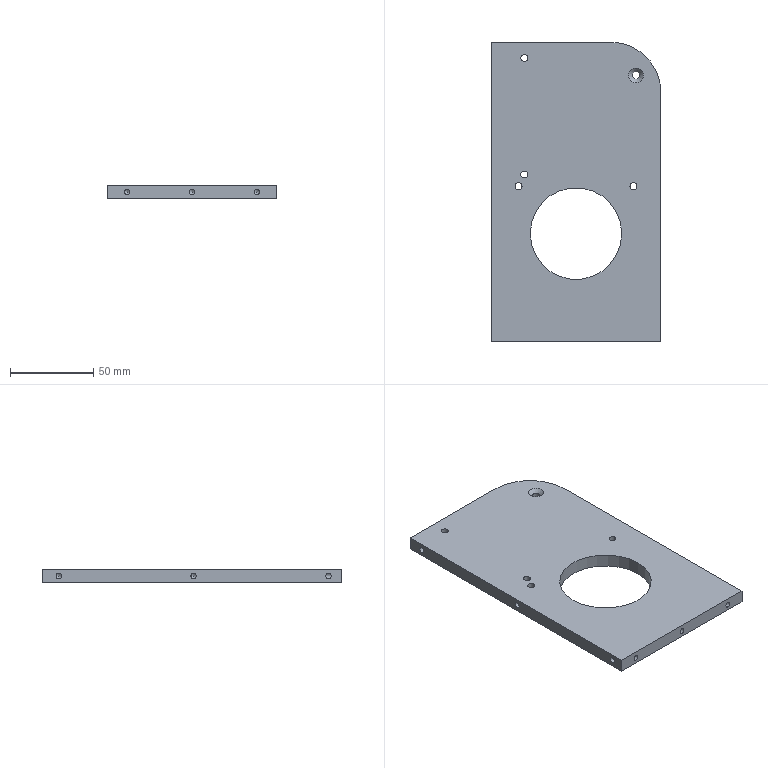Part | NX | 1 solid | 36 faces | box 102 x 180 x 8 mm | volume 124761 mm3 | cylinder 18 | cone 12 | plane 6 | commonest cylinder face diameters 3.3 x11 4.2 x4 4.5 x1 55 x1 60 x1
STEP:
#1=CARTESIAN_POINT('',(39.5,-130.5,-1.572));
#2=VERTEX_POINT('',#1);
#3=CARTESIAN_POINT('',(39.5,-129.5,-1.572));
#4=VERTEX_POINT('',#3);
#5=CARTESIAN_POINT('',(39.5,-130.,0.));
#6=DIRECTION('',(1.,0.,0.));
#7=DIRECTION('',(0.,0.,-1.));
#8=AXIS2_PLACEMENT_3D('',#5,#6,#7);
#9=CIRCLE('',#8,1.65);
#10=EDGE_CURVE('',#2,#4,#9,.T.);
#11=ORIENTED_EDGE('',*,*,#10,.T.);
#12=CARTESIAN_POINT('',(39.5,-129.5,-1.572));
#13=CARTESIAN_POINT('',(39.449,-129.829,-1.589));
#14=CARTESIAN_POINT('',(39.449,-130.17,-1.589));
#15=CARTESIAN_POINT('',(39.5,-130.5,-1.572));
#16=B_SPLINE_CURVE_WITH_KNOTS('',3,(#12,#13,#14,#15),.UNSPECIFIED.,.F.,.F.,(4,4),(0.000476,0.001477),.UNSPECIFIED.);
#17=EDGE_CURVE('',#4,#2,#16,.T.);
#18=ORIENTED_EDGE('',*,*,#17,.T.);
#19=EDGE_LOOP('',(#11,#18));
#20=FACE_BOUND('',#19,.T.);
#21=CARTESIAN_POINT('',(39.5,-130.,0.));
#22=DIRECTION('',(1.,0.,0.));
#23=DIRECTION('',(0.,0.,-1.));
#24=AXIS2_PLACEMENT_3D('',#21,#22,#23);
#25=CONICAL_SURFACE('',#24,1.65,1.03);
#26=ADVANCED_FACE('',(#20),#25,.F.);
#27=CARTESIAN_POINT('',(-39.5,-132.5,1.572));
#28=VERTEX_POINT('',#27);
#29=CARTESIAN_POINT('',(-39.5,-131.5,1.572));
#30=VERTEX_POINT('',#29);
#31=CARTESIAN_POINT('',(-39.5,-132.,0.));
#32=DIRECTION('',(-1.,0.,0.));
#33=DIRECTION('',(0.,0.,1.));
#34=AXIS2_PLACEMENT_3D('',#31,#32,#33);
#35=CIRCLE('',#34,1.65);
#36=EDGE_CURVE('',#28,#30,#35,.T.);
#37=ORIENTED_EDGE('',*,*,#36,.T.);
#38=CARTESIAN_POINT('',(-39.5,-131.5,1.572));
#39=CARTESIAN_POINT('',(-39.449,-131.829,1.589));
#40=CARTESIAN_POINT('',(-39.449,-132.17,1.589));
#41=CARTESIAN_POINT('',(-39.5,-132.5,1.572));
#42=B_SPLINE_CURVE_WITH_KNOTS('',3,(#38,#39,#40,#41),.UNSPECIFIED.,.F.,.F.,(4,4),(0.000476,0.001477),.UNSPECIFIED.);
#43=EDGE_CURVE('',#30,#28,#42,.T.);
#44=ORIENTED_EDGE('',*,*,#43,.T.);
#45=EDGE_LOOP('',(#37,#44));
#46=FACE_BOUND('',#45,.T.);
#47=CARTESIAN_POINT('',(-39.5,-132.,0.));
#48=DIRECTION('',(-1.,0.,0.));
#49=DIRECTION('',(0.,0.,1.));
#50=AXIS2_PLACEMENT_3D('',#47,#48,#49);
#51=CONICAL_SURFACE('',#50,1.65,1.03);
#52=ADVANCED_FACE('',(#46),#51,.F.);
#53=CARTESIAN_POINT('',(-28.9,30.505,4.));
#54=VERTEX_POINT('',#53);
#55=CARTESIAN_POINT('',(-31.,30.505,4.));
#56=DIRECTION('',(0.,0.,1.));
#57=DIRECTION('',(1.,0.,0.));
#58=AXIS2_PLACEMENT_3D('',#55,#56,#57);
#59=CIRCLE('',#58,2.1);
#60=EDGE_CURVE('',#54,#54,#59,.T.);
#61=ORIENTED_EDGE('',*,*,#60,.F.);
#62=EDGE_LOOP('',(#61));
#63=FACE_BOUND('',#62,.T.);
#64=CARTESIAN_POINT('',(-28.9,-39.495,4.));
#65=VERTEX_POINT('',#64);
#66=CARTESIAN_POINT('',(-31.,-39.495,4.));
#67=DIRECTION('',(0.,0.,1.));
#68=DIRECTION('',(1.,0.,0.));
#69=AXIS2_PLACEMENT_3D('',#66,#67,#68);
#70=CIRCLE('',#69,2.1);
#71=EDGE_CURVE('',#65,#65,#70,.T.);
#72=ORIENTED_EDGE('',*,*,#71,.F.);
#73=EDGE_LOOP('',(#72));
#74=FACE_BOUND('',#73,.T.);
#75=CARTESIAN_POINT('',(36.6,-46.5,4.));
#76=VERTEX_POINT('',#75);
#77=CARTESIAN_POINT('',(34.5,-46.5,4.));
#78=DIRECTION('',(0.,0.,1.));
#79=DIRECTION('',(1.,0.,0.));
#80=AXIS2_PLACEMENT_3D('',#77,#78,#79);
#81=CIRCLE('',#80,2.1);
#82=EDGE_CURVE('',#76,#76,#81,.T.);
#83=ORIENTED_EDGE('',*,*,#82,.F.);
#84=EDGE_LOOP('',(#83));
#85=FACE_BOUND('',#84,.T.);
#86=CARTESIAN_POINT('',(-32.4,-46.5,4.));
#87=VERTEX_POINT('',#86);
#88=CARTESIAN_POINT('',(-34.5,-46.5,4.));
#89=DIRECTION('',(0.,0.,1.));
#90=DIRECTION('',(1.,0.,0.));
#91=AXIS2_PLACEMENT_3D('',#88,#89,#90);
#92=CIRCLE('',#91,2.1);
#93=EDGE_CURVE('',#87,#87,#92,.T.);
#94=ORIENTED_EDGE('',*,*,#93,.F.);
#95=EDGE_LOOP('',(#94));
#96=FACE_BOUND('',#95,.T.);
#97=CARTESIAN_POINT('',(40.5,20.,4.));
#98=VERTEX_POINT('',#97);
#99=CARTESIAN_POINT('',(36.,20.,4.));
#100=DIRECTION('',(0.,0.,1.));
#101=DIRECTION('',(1.,0.,0.));
#102=AXIS2_PLACEMENT_3D('',#99,#100,#101);
#103=CIRCLE('',#102,4.5);
#104=EDGE_CURVE('',#98,#98,#103,.T.);
#105=ORIENTED_EDGE('',*,*,#104,.F.);
#106=EDGE_LOOP('',(#105));
#107=FACE_BOUND('',#106,.T.);
#108=CARTESIAN_POINT('',(51.,-140.,4.));
#109=VERTEX_POINT('',#108);
#110=CARTESIAN_POINT('',(51.,10.,4.));
#111=VERTEX_POINT('',#110);
#112=CARTESIAN_POINT('',(51.,40.,4.));
#113=DIRECTION('',(0.,1.,0.));
#114=VECTOR('',#113,1000.);
#115=LINE('',#112,#114);
#116=EDGE_CURVE('',#109,#111,#115,.T.);
#117=ORIENTED_EDGE('',*,*,#116,.T.);
#118=CARTESIAN_POINT('',(21.,40.,4.));
#119=VERTEX_POINT('',#118);
#120=CARTESIAN_POINT('',(21.,10.,4.));
#121=DIRECTION('',(0.,0.,1.));
#122=DIRECTION('',(1.,0.,0.));
#123=AXIS2_PLACEMENT_3D('',#120,#121,#122);
#124=CIRCLE('',#123,30.);
#125=EDGE_CURVE('',#111,#119,#124,.T.);
#126=ORIENTED_EDGE('',*,*,#125,.T.);
#127=CARTESIAN_POINT('',(-51.,40.,4.));
#128=VERTEX_POINT('',#127);
#129=CARTESIAN_POINT('',(-51.,40.,4.));
#130=DIRECTION('',(-1.,0.,0.));
#131=VECTOR('',#130,1000.);
#132=LINE('',#129,#131);
#133=EDGE_CURVE('',#119,#128,#132,.T.);
#134=ORIENTED_EDGE('',*,*,#133,.T.);
#135=CARTESIAN_POINT('',(-51.,-140.,4.));
#136=VERTEX_POINT('',#135);
#137=CARTESIAN_POINT('',(-51.,40.,4.));
#138=DIRECTION('',(0.,-1.,0.));
#139=VECTOR('',#138,1000.);
#140=LINE('',#137,#139);
#141=EDGE_CURVE('',#128,#136,#140,.T.);
#142=ORIENTED_EDGE('',*,*,#141,.T.);
#143=CARTESIAN_POINT('',(51.,-140.,4.));
#144=DIRECTION('',(-1.,0.,0.));
#145=VECTOR('',#144,1000.);
#146=LINE('',#143,#145);
#147=EDGE_CURVE('',#109,#136,#146,.T.);
#148=ORIENTED_EDGE('',*,*,#147,.F.);
#149=EDGE_LOOP('',(#117,#126,#134,#142,#148));
#150=FACE_BOUND('',#149,.T.);
#151=CARTESIAN_POINT('',(-27.5,-75.,4.));
#152=VERTEX_POINT('',#151);
#153=CARTESIAN_POINT('',(0.,-75.,4.));
#154=DIRECTION('',(0.,0.,-1.));
#155=DIRECTION('',(-1.,0.,0.));
#156=AXIS2_PLACEMENT_3D('',#153,#154,#155);
#157=CIRCLE('',#156,27.5);
#158=EDGE_CURVE('',#152,#152,#157,.T.);
#159=ORIENTED_EDGE('',*,*,#158,.T.);
#160=EDGE_LOOP('',(#159));
#161=FACE_BOUND('',#160,.T.);
#162=CARTESIAN_POINT('',(0.,0.,4.));
#163=DIRECTION('',(0.,0.,1.));
#164=DIRECTION('',(1.,0.,0.));
#165=AXIS2_PLACEMENT_3D('',#162,#163,#164);
#166=PLANE('',#165);
#167=ADVANCED_FACE('',(#63,#74,#85,#96,#107,#150,#161),#166,.T.);
#168=CARTESIAN_POINT('',(-28.9,30.505,-4.));
#169=VERTEX_POINT('',#168);
#170=CARTESIAN_POINT('',(-31.,30.505,-4.));
#171=DIRECTION('',(0.,0.,1.));
#172=DIRECTION('',(1.,0.,0.));
#173=AXIS2_PLACEMENT_3D('',#170,#171,#172);
#174=CIRCLE('',#173,2.1);
#175=EDGE_CURVE('',#169,#169,#174,.T.);
#176=ORIENTED_EDGE('',*,*,#175,.T.);
#177=EDGE_LOOP('',(#176));
#178=FACE_BOUND('',#177,.T.);
#179=CARTESIAN_POINT('',(-28.9,-39.495,-4.));
#180=VERTEX_POINT('',#179);
#181=CARTESIAN_POINT('',(-31.,-39.495,-4.));
#182=DIRECTION('',(0.,0.,1.));
#183=DIRECTION('',(1.,0.,0.));
#184=AXIS2_PLACEMENT_3D('',#181,#182,#183);
#185=CIRCLE('',#184,2.1);
#186=EDGE_CURVE('',#180,#180,#185,.T.);
#187=ORIENTED_EDGE('',*,*,#186,.T.);
#188=EDGE_LOOP('',(#187));
#189=FACE_BOUND('',#188,.T.);
#190=CARTESIAN_POINT('',(36.6,-46.5,-4.));
#191=VERTEX_POINT('',#190);
#192=CARTESIAN_POINT('',(34.5,-46.5,-4.));
#193=DIRECTION('',(0.,0.,1.));
#194=DIRECTION('',(1.,0.,0.));
#195=AXIS2_PLACEMENT_3D('',#192,#193,#194);
#196=CIRCLE('',#195,2.1);
#197=EDGE_CURVE('',#191,#191,#196,.T.);
#198=ORIENTED_EDGE('',*,*,#197,.T.);
#199=EDGE_LOOP('',(#198));
#200=FACE_BOUND('',#199,.T.);
#201=CARTESIAN_POINT('',(-32.4,-46.5,-4.));
#202=VERTEX_POINT('',#201);
#203=CARTESIAN_POINT('',(-34.5,-46.5,-4.));
#204=DIRECTION('',(0.,0.,1.));
#205=DIRECTION('',(1.,0.,0.));
#206=AXIS2_PLACEMENT_3D('',#203,#204,#205);
#207=CIRCLE('',#206,2.1);
#208=EDGE_CURVE('',#202,#202,#207,.T.);
#209=ORIENTED_EDGE('',*,*,#208,.T.);
#210=EDGE_LOOP('',(#209));
#211=FACE_BOUND('',#210,.T.);
#212=CARTESIAN_POINT('',(38.25,20.,-4.));
#213=VERTEX_POINT('',#212);
#214=CARTESIAN_POINT('',(36.,20.,-4.));
#215=DIRECTION('',(0.,0.,1.));
#216=DIRECTION('',(1.,0.,0.));
#217=AXIS2_PLACEMENT_3D('',#214,#215,#216);
#218=CIRCLE('',#217,2.25);
#219=EDGE_CURVE('',#213,#213,#218,.T.);
#220=ORIENTED_EDGE('',*,*,#219,.T.);
#221=EDGE_LOOP('',(#220));
#222=FACE_BOUND('',#221,.T.);
#223=CARTESIAN_POINT('',(21.,40.,-4.));
#224=VERTEX_POINT('',#223);
#225=CARTESIAN_POINT('',(-51.,40.,-4.));
#226=VERTEX_POINT('',#225);
#227=CARTESIAN_POINT('',(-51.,40.,-4.));
#228=DIRECTION('',(-1.,0.,0.));
#229=VECTOR('',#228,1000.);
#230=LINE('',#227,#229);
#231=EDGE_CURVE('',#224,#226,#230,.T.);
#232=ORIENTED_EDGE('',*,*,#231,.F.);
#233=CARTESIAN_POINT('',(51.,10.,-4.));
#234=VERTEX_POINT('',#233);
#235=CARTESIAN_POINT('',(21.,10.,-4.));
#236=DIRECTION('',(0.,0.,1.));
#237=DIRECTION('',(1.,0.,0.));
#238=AXIS2_PLACEMENT_3D('',#235,#236,#237);
#239=CIRCLE('',#238,30.);
#240=EDGE_CURVE('',#224,#234,#239,.F.);
#241=ORIENTED_EDGE('',*,*,#240,.T.);
#242=CARTESIAN_POINT('',(51.,-140.,-4.));
#243=VERTEX_POINT('',#242);
#244=CARTESIAN_POINT('',(51.,40.,-4.));
#245=DIRECTION('',(0.,1.,0.));
#246=VECTOR('',#245,1000.);
#247=LINE('',#244,#246);
#248=EDGE_CURVE('',#243,#234,#247,.T.);
#249=ORIENTED_EDGE('',*,*,#248,.F.);
#250=CARTESIAN_POINT('',(-51.,-140.,-4.));
#251=VERTEX_POINT('',#250);
#252=CARTESIAN_POINT('',(51.,-140.,-4.));
#253=DIRECTION('',(1.,0.,0.));
#254=VECTOR('',#253,1000.);
#255=LINE('',#252,#254);
#256=EDGE_CURVE('',#251,#243,#255,.T.);
#257=ORIENTED_EDGE('',*,*,#256,.F.);
#258=CARTESIAN_POINT('',(-51.,40.,-4.));
#259=DIRECTION('',(0.,-1.,0.));
#260=VECTOR('',#259,1000.);
#261=LINE('',#258,#260);
#262=EDGE_CURVE('',#226,#251,#261,.T.);
#263=ORIENTED_EDGE('',*,*,#262,.F.);
#264=EDGE_LOOP('',(#232,#241,#249,#257,#263));
#265=FACE_BOUND('',#264,.T.);
#266=CARTESIAN_POINT('',(-27.5,-75.,-4.));
#267=VERTEX_POINT('',#266);
#268=CARTESIAN_POINT('',(0.,-75.,-4.));
#269=DIRECTION('',(0.,0.,-1.));
#270=DIRECTION('',(-1.,0.,0.));
#271=AXIS2_PLACEMENT_3D('',#268,#269,#270);
#272=CIRCLE('',#271,27.5);
#273=EDGE_CURVE('',#267,#267,#272,.T.);
#274=ORIENTED_EDGE('',*,*,#273,.F.);
#275=EDGE_LOOP('',(#274));
#276=FACE_BOUND('',#275,.T.);
#277=CARTESIAN_POINT('',(0.,0.,-4.));
#278=DIRECTION('',(0.,0.,1.));
#279=DIRECTION('',(1.,0.,0.));
#280=AXIS2_PLACEMENT_3D('',#277,#278,#279);
#281=PLANE('',#280);
#282=ADVANCED_FACE('',(#178,#189,#200,#211,#222,#265,#276),#281,.F.);
#283=CARTESIAN_POINT('',(51.,5.,-1.65));
#284=VERTEX_POINT('',#283);
#285=CARTESIAN_POINT('',(51.,5.,0.));
#286=DIRECTION('',(1.,0.,0.));
#287=DIRECTION('',(0.,0.,-1.));
#288=AXIS2_PLACEMENT_3D('',#285,#286,#287);
#289=CIRCLE('',#288,1.65);
#290=EDGE_CURVE('',#284,#284,#289,.T.);
#291=ORIENTED_EDGE('',*,*,#290,.F.);
#292=EDGE_LOOP('',(#291));
#293=FACE_BOUND('',#292,.T.);
#294=CARTESIAN_POINT('',(51.,-130.,-1.65));
#295=VERTEX_POINT('',#294);
#296=CARTESIAN_POINT('',(51.,-130.,0.));
#297=DIRECTION('',(1.,0.,0.));
#298=DIRECTION('',(0.,0.,-1.));
#299=AXIS2_PLACEMENT_3D('',#296,#297,#298);
#300=CIRCLE('',#299,1.65);
#301=EDGE_CURVE('',#295,#295,#300,.T.);
#302=ORIENTED_EDGE('',*,*,#301,.F.);
#303=EDGE_LOOP('',(#302));
#304=FACE_BOUND('',#303,.T.);
#305=ORIENTED_EDGE('',*,*,#248,.T.);
#306=CARTESIAN_POINT('',(51.,10.,4.));
#307=DIRECTION('',(0.,0.,-1.));
#308=VECTOR('',#307,1000.);
#309=LINE('',#306,#308);
#310=EDGE_CURVE('',#234,#111,#309,.F.);
#311=ORIENTED_EDGE('',*,*,#310,.T.);
#312=ORIENTED_EDGE('',*,*,#116,.F.);
#313=CARTESIAN_POINT('',(51.,-140.,-146.843));
#314=DIRECTION('',(0.,0.,1.));
#315=VECTOR('',#314,1000.);
#316=LINE('',#313,#315);
#317=EDGE_CURVE('',#243,#109,#316,.T.);
#318=ORIENTED_EDGE('',*,*,#317,.F.);
#319=EDGE_LOOP('',(#305,#311,#312,#318));
#320=FACE_BOUND('',#319,.T.);
#321=CARTESIAN_POINT('',(51.,40.,4.));
#322=DIRECTION('',(-1.,0.,0.));
#323=DIRECTION('',(0.,0.,1.));
#324=AXIS2_PLACEMENT_3D('',#321,#322,#323);
#325=PLANE('',#324);
#326=ADVANCED_FACE('',(#293,#304,#320),#325,.F.);
#327=CARTESIAN_POINT('',(-31.,40.,1.65));
#328=VERTEX_POINT('',#327);
#329=CARTESIAN_POINT('',(-31.,40.,0.));
#330=DIRECTION('',(0.,1.,0.));
#331=DIRECTION('',(0.,0.,1.));
#332=AXIS2_PLACEMENT_3D('',#329,#330,#331);
#333=CIRCLE('',#332,1.65);
#334=EDGE_CURVE('',#328,#328,#333,.T.);
#335=ORIENTED_EDGE('',*,*,#334,.F.);
#336=EDGE_LOOP('',(#335));
#337=FACE_BOUND('',#336,.T.);
#338=ORIENTED_EDGE('',*,*,#133,.F.);
#339=CARTESIAN_POINT('',(21.,40.,4.));
#340=DIRECTION('',(0.,0.,-1.));
#341=VECTOR('',#340,1000.);
#342=LINE('',#339,#341);
#343=EDGE_CURVE('',#119,#224,#342,.T.);
#344=ORIENTED_EDGE('',*,*,#343,.T.);
#345=ORIENTED_EDGE('',*,*,#231,.T.);
#346=CARTESIAN_POINT('',(-51.,40.,4.));
#347=DIRECTION('',(0.,0.,-1.));
#348=VECTOR('',#347,1000.);
#349=LINE('',#346,#348);
#350=EDGE_CURVE('',#128,#226,#349,.T.);
#351=ORIENTED_EDGE('',*,*,#350,.F.);
#352=EDGE_LOOP('',(#338,#344,#345,#351));
#353=FACE_BOUND('',#352,.T.);
#354=CARTESIAN_POINT('',(-51.,40.,4.));
#355=DIRECTION('',(0.,-1.,0.));
#356=DIRECTION('',(0.,0.,-1.));
#357=AXIS2_PLACEMENT_3D('',#354,#355,#356);
#358=PLANE('',#357);
#359=ADVANCED_FACE('',(#337,#353),#358,.F.);
#360=CARTESIAN_POINT('',(-51.,30.,1.65));
#361=VERTEX_POINT('',#360);
#362=CARTESIAN_POINT('',(-51.,30.,0.));
#363=DIRECTION('',(-1.,0.,0.));
#364=DIRECTION('',(0.,0.,1.));
#365=AXIS2_PLACEMENT_3D('',#362,#363,#364);
#366=CIRCLE('',#365,1.65);
#367=EDGE_CURVE('',#361,#361,#366,.T.);
#368=ORIENTED_EDGE('',*,*,#367,.F.);
#369=EDGE_LOOP('',(#368));
#370=FACE_BOUND('',#369,.T.);
#371=CARTESIAN_POINT('',(-51.,-51.,1.65));
#372=VERTEX_POINT('',#371);
#373=CARTESIAN_POINT('',(-51.,-51.,0.));
#374=DIRECTION('',(-1.,0.,0.));
#375=DIRECTION('',(0.,0.,1.));
#376=AXIS2_PLACEMENT_3D('',#373,#374,#375);
#377=CIRCLE('',#376,1.65);
#378=EDGE_CURVE('',#372,#372,#377,.T.);
#379=ORIENTED_EDGE('',*,*,#378,.F.);
#380=EDGE_LOOP('',(#379));
#381=FACE_BOUND('',#380,.T.);
#382=CARTESIAN_POINT('',(-51.,-132.,1.65));
#383=VERTEX_POINT('',#382);
#384=CARTESIAN_POINT('',(-51.,-132.,0.));
#385=DIRECTION('',(-1.,0.,0.));
#386=DIRECTION('',(0.,0.,1.));
#387=AXIS2_PLACEMENT_3D('',#384,#385,#386);
#388=CIRCLE('',#387,1.65);
#389=EDGE_CURVE('',#383,#383,#388,.T.);
#390=ORIENTED_EDGE('',*,*,#389,.F.);
#391=EDGE_LOOP('',(#390));
#392=FACE_BOUND('',#391,.T.);
#393=ORIENTED_EDGE('',*,*,#262,.T.);
#394=CARTESIAN_POINT('',(-51.,-140.,-146.843));
#395=DIRECTION('',(0.,0.,1.));
#396=VECTOR('',#395,1000.);
#397=LINE('',#394,#396);
#398=EDGE_CURVE('',#251,#136,#397,.T.);
#399=ORIENTED_EDGE('',*,*,#398,.T.);
#400=ORIENTED_EDGE('',*,*,#141,.F.);
#401=ORIENTED_EDGE('',*,*,#350,.T.);
#402=EDGE_LOOP('',(#393,#399,#400,#401));
#403=FACE_BOUND('',#402,.T.);
#404=CARTESIAN_POINT('',(-51.,40.,4.));
#405=DIRECTION('',(1.,0.,0.));
#406=DIRECTION('',(0.,1.,0.));
#407=AXIS2_PLACEMENT_3D('',#404,#405,#406);
#408=PLANE('',#407);
#409=ADVANCED_FACE('',(#370,#381,#392,#403),#408,.F.);
#410=CARTESIAN_POINT('',(39.,-140.,-1.65));
#411=VERTEX_POINT('',#410);
#412=CARTESIAN_POINT('',(39.,-140.,0.));
#413=DIRECTION('',(0.,-1.,0.));
#414=DIRECTION('',(0.,0.,-1.));
#415=AXIS2_PLACEMENT_3D('',#412,#413,#414);
#416=CIRCLE('',#415,1.65);
#417=EDGE_CURVE('',#411,#411,#416,.T.);
#418=ORIENTED_EDGE('',*,*,#417,.F.);
#419=EDGE_LOOP('',(#418));
#420=FACE_BOUND('',#419,.T.);
#421=CARTESIAN_POINT('',(0.,-140.,-1.65));
#422=VERTEX_POINT('',#421);
#423=CARTESIAN_POINT('',(0.,-140.,0.));
#424=DIRECTION('',(0.,-1.,0.));
#425=DIRECTION('',(0.,0.,-1.));
#426=AXIS2_PLACEMENT_3D('',#423,#424,#425);
#427=CIRCLE('',#426,1.65);
#428=EDGE_CURVE('',#422,#422,#427,.T.);
#429=ORIENTED_EDGE('',*,*,#428,.F.);
#430=EDGE_LOOP('',(#429));
#431=FACE_BOUND('',#430,.T.);
#432=CARTESIAN_POINT('',(-39.,-140.,-1.65));
#433=VERTEX_POINT('',#432);
#434=CARTESIAN_POINT('',(-39.,-140.,0.));
#435=DIRECTION('',(0.,-1.,0.));
#436=DIRECTION('',(0.,0.,-1.));
#437=AXIS2_PLACEMENT_3D('',#434,#435,#436);
#438=CIRCLE('',#437,1.65);
#439=EDGE_CURVE('',#433,#433,#438,.T.);
#440=ORIENTED_EDGE('',*,*,#439,.F.);
#441=EDGE_LOOP('',(#440));
#442=FACE_BOUND('',#441,.T.);
#443=ORIENTED_EDGE('',*,*,#398,.F.);
#444=ORIENTED_EDGE('',*,*,#256,.T.);
#445=ORIENTED_EDGE('',*,*,#317,.T.);
#446=ORIENTED_EDGE('',*,*,#147,.T.);
#447=EDGE_LOOP('',(#443,#444,#445,#446));
#448=FACE_BOUND('',#447,.T.);
#449=CARTESIAN_POINT('',(51.,-140.,-146.843));
#450=DIRECTION('',(0.,1.,0.));
#451=DIRECTION('',(0.,0.,1.));
#452=AXIS2_PLACEMENT_3D('',#449,#450,#451);
#453=PLANE('',#452);
#454=ADVANCED_FACE('',(#420,#431,#442,#448),#453,.F.);
#455=ORIENTED_EDGE('',*,*,#273,.T.);
#456=EDGE_LOOP('',(#455));
#457=FACE_BOUND('',#456,.T.);
#458=ORIENTED_EDGE('',*,*,#158,.F.);
#459=EDGE_LOOP('',(#458));
#460=FACE_BOUND('',#459,.T.);
#461=CARTESIAN_POINT('',(0.,-75.,-4.));
#462=DIRECTION('',(0.,0.,1.));
#463=DIRECTION('',(1.,0.,0.));
#464=AXIS2_PLACEMENT_3D('',#461,#462,#463);
#465=CYLINDRICAL_SURFACE('',#464,27.5);
#466=ADVANCED_FACE('',(#457,#460),#465,.F.);
#467=CARTESIAN_POINT('',(-39.5,-131.5,-1.572));
#468=VERTEX_POINT('',#467);
#469=CARTESIAN_POINT('',(-39.5,-132.5,-1.572));
#470=VERTEX_POINT('',#469);
#471=CARTESIAN_POINT('',(-39.5,-132.,0.));
#472=DIRECTION('',(-1.,0.,0.));
#473=DIRECTION('',(0.,0.,1.));
#474=AXIS2_PLACEMENT_3D('',#471,#472,#473);
#475=CIRCLE('',#474,1.65);
#476=EDGE_CURVE('',#468,#470,#475,.T.);
#477=ORIENTED_EDGE('',*,*,#476,.T.);
#478=CARTESIAN_POINT('',(-39.5,-132.5,-1.572));
#479=CARTESIAN_POINT('',(-39.449,-132.171,-1.589));
#480=CARTESIAN_POINT('',(-39.449,-131.83,-1.589));
#481=CARTESIAN_POINT('',(-39.5,-131.5,-1.572));
#482=B_SPLINE_CURVE_WITH_KNOTS('',3,(#478,#479,#480,#481),.UNSPECIFIED.,.F.,.F.,(4,4),(0.000476,0.001477),.UNSPECIFIED.);
#483=EDGE_CURVE('',#470,#468,#482,.T.);
#484=ORIENTED_EDGE('',*,*,#483,.T.);
#485=EDGE_LOOP('',(#477,#484));
#486=FACE_BOUND('',#485,.T.);
#487=CARTESIAN_POINT('',(-39.5,-132.,0.));
#488=DIRECTION('',(-1.,0.,0.));
#489=DIRECTION('',(0.,0.,1.));
#490=AXIS2_PLACEMENT_3D('',#487,#488,#489);
#491=CONICAL_SURFACE('',#490,1.65,1.03);
#492=ADVANCED_FACE('',(#486),#491,.F.);
#493=ORIENTED_EDGE('',*,*,#476,.F.);
#494=CARTESIAN_POINT('',(-39.,-132.,0.));
#495=DIRECTION('',(-0.7071,-0.7071,0.));
#496=DIRECTION('',(-0.7071,0.7071,0.));
#497=AXIS2_PLACEMENT_3D('',#494,#495,#496);
#498=ELLIPSE('',#497,2.333,1.65);
#499=EDGE_CURVE('',#468,#30,#498,.F.);
#500=ORIENTED_EDGE('',*,*,#499,.T.);
#501=ORIENTED_EDGE('',*,*,#36,.F.);
#502=CARTESIAN_POINT('',(-39.,-132.,0.));
#503=DIRECTION('',(-0.7071,0.7071,0.));
#504=DIRECTION('',(-0.7071,-0.7071,0.));
#505=AXIS2_PLACEMENT_3D('',#502,#503,#504);
#506=ELLIPSE('',#505,2.333,1.65);
#507=EDGE_CURVE('',#28,#470,#506,.F.);
#508=ORIENTED_EDGE('',*,*,#507,.T.);
#509=EDGE_LOOP('',(#493,#500,#501,#508));
#510=FACE_BOUND('',#509,.T.);
#511=ORIENTED_EDGE('',*,*,#389,.T.);
#512=EDGE_LOOP('',(#511));
#513=FACE_BOUND('',#512,.T.);
#514=CARTESIAN_POINT('',(-51.,-132.,0.));
#515=DIRECTION('',(-1.,0.,0.));
#516=DIRECTION('',(0.,0.,1.));
#517=AXIS2_PLACEMENT_3D('',#514,#515,#516);
#518=CYLINDRICAL_SURFACE('',#517,1.65);
#519=ADVANCED_FACE('',(#510,#513),#518,.F.);
#520=CARTESIAN_POINT('',(-38.509,-51.,0.));
#521=VERTEX_POINT('',#520);
#522=VERTEX_LOOP('',#521);
#523=FACE_BOUND('',#522,.T.);
#524=CARTESIAN_POINT('',(-39.5,-51.,1.65));
#525=VERTEX_POINT('',#524);
#526=CARTESIAN_POINT('',(-39.5,-51.,0.));
#527=DIRECTION('',(-1.,0.,0.));
#528=DIRECTION('',(0.,0.,1.));
#529=AXIS2_PLACEMENT_3D('',#526,#527,#528);
#530=CIRCLE('',#529,1.65);
#531=EDGE_CURVE('',#525,#525,#530,.T.);
#532=ORIENTED_EDGE('',*,*,#531,.T.);
#533=EDGE_LOOP('',(#532));
#534=FACE_BOUND('',#533,.T.);
#535=CARTESIAN_POINT('',(-39.5,-51.,0.));
#536=DIRECTION('',(-1.,0.,0.));
#537=DIRECTION('',(0.,0.,1.));
#538=AXIS2_PLACEMENT_3D('',#535,#536,#537);
#539=CONICAL_SURFACE('',#538,1.65,1.03);
#540=ADVANCED_FACE('',(#523,#534),#539,.F.);
#541=ORIENTED_EDGE('',*,*,#531,.F.);
#542=EDGE_LOOP('',(#541));
#543=FACE_BOUND('',#542,.T.);
#544=ORIENTED_EDGE('',*,*,#378,.T.);
#545=EDGE_LOOP('',(#544));
#546=FACE_BOUND('',#545,.T.);
#547=CARTESIAN_POINT('',(-51.,-51.,0.));
#548=DIRECTION('',(-1.,0.,0.));
#549=DIRECTION('',(0.,0.,1.));
#550=AXIS2_PLACEMENT_3D('',#547,#548,#549);
#551=CYLINDRICAL_SURFACE('',#550,1.65);
#552=ADVANCED_FACE('',(#543,#546),#551,.F.);
#553=CARTESIAN_POINT('',(-38.509,30.,0.));
#554=VERTEX_POINT('',#553);
#555=VERTEX_LOOP('',#554);
#556=FACE_BOUND('',#555,.T.);
#557=CARTESIAN_POINT('',(-39.5,30.,1.65));
#558=VERTEX_POINT('',#557);
#559=CARTESIAN_POINT('',(-39.5,30.,0.));
#560=DIRECTION('',(-1.,0.,0.));
#561=DIRECTION('',(0.,0.,1.));
#562=AXIS2_PLACEMENT_3D('',#559,#560,#561);
#563=CIRCLE('',#562,1.65);
#564=EDGE_CURVE('',#558,#558,#563,.T.);
#565=ORIENTED_EDGE('',*,*,#564,.T.);
#566=EDGE_LOOP('',(#565));
#567=FACE_BOUND('',#566,.T.);
#568=CARTESIAN_POINT('',(-39.5,30.,0.));
#569=DIRECTION('',(-1.,0.,0.));
#570=DIRECTION('',(0.,0.,1.));
#571=AXIS2_PLACEMENT_3D('',#568,#569,#570);
#572=CONICAL_SURFACE('',#571,1.65,1.03);
#573=ADVANCED_FACE('',(#556,#567),#572,.F.);
#574=ORIENTED_EDGE('',*,*,#564,.F.);
#575=EDGE_LOOP('',(#574));
#576=FACE_BOUND('',#575,.T.);
#577=ORIENTED_EDGE('',*,*,#367,.T.);
#578=EDGE_LOOP('',(#577));
#579=FACE_BOUND('',#578,.T.);
#580=CARTESIAN_POINT('',(-51.,30.,0.));
#581=DIRECTION('',(-1.,0.,0.));
#582=DIRECTION('',(0.,0.,1.));
#583=AXIS2_PLACEMENT_3D('',#580,#581,#582);
#584=CYLINDRICAL_SURFACE('',#583,1.65);
#585=ADVANCED_FACE('',(#576,#579),#584,.F.);
#586=CARTESIAN_POINT('',(-31.,32.605,1.65));
#587=VERTEX_POINT('',#586);
#588=CARTESIAN_POINT('',(-29.691,32.284,1.274));
#589=CARTESIAN_POINT('',(-30.998,32.767,1.844));
#590=CARTESIAN_POINT('',(-32.097,32.36,1.35));
#591=CARTESIAN_POINT('',(-32.549,31.937,0.6794));
#592=CARTESIAN_POINT('',(-32.744,31.677,-0.2313));
#593=CARTESIAN_POINT('',(-32.308,32.285,-1.267));
#594=CARTESIAN_POINT('',(-31.01,32.764,-1.838));
#595=CARTESIAN_POINT('',(-29.693,32.289,-1.281));
#596=CARTESIAN_POINT('',(-29.179,31.563,-0.0006032));
#597=CARTESIAN_POINT('',(-29.691,32.284,1.274));
#598=CARTESIAN_POINT('',(-30.998,32.767,1.844));
#599=CARTESIAN_POINT('',(-32.097,32.36,1.35));
#600=B_SPLINE_CURVE_WITH_KNOTS('',3,(#588,#589,#590,#591,#592,#593,#594,#595,#596,#597,#598,#599),.UNSPECIFIED.,.T.,.F.,(1,1,1,1,1,1,1,1,1,1,1,1,1,1,1,1),(-0.00408,-0.00272,-0.00136,0.,0.00136,0.00204,0.00272,0.00408,0.00544,0.006799,0.008159,0.009519,0.01088,0.01224,0.01292,0.0136),.UNSPECIFIED.);
#601=EDGE_CURVE('',#587,#587,#600,.T.);
#602=ORIENTED_EDGE('',*,*,#601,.T.);
#603=EDGE_LOOP('',(#602));
#604=FACE_BOUND('',#603,.T.);
#605=ORIENTED_EDGE('',*,*,#334,.T.);
#606=EDGE_LOOP('',(#605));
#607=FACE_BOUND('',#606,.T.);
#608=CARTESIAN_POINT('',(-31.,40.,0.));
#609=DIRECTION('',(0.,1.,0.));
#610=DIRECTION('',(0.,0.,1.));
#611=AXIS2_PLACEMENT_3D('',#608,#609,#610);
#612=CYLINDRICAL_SURFACE('',#611,1.65);
#613=ADVANCED_FACE('',(#604,#607),#612,.F.);
#614=CARTESIAN_POINT('',(39.5,-129.5,1.572));
#615=VERTEX_POINT('',#614);
#616=CARTESIAN_POINT('',(39.5,-130.5,1.572));
#617=VERTEX_POINT('',#616);
#618=CARTESIAN_POINT('',(39.5,-130.,0.));
#619=DIRECTION('',(1.,0.,0.));
#620=DIRECTION('',(0.,0.,-1.));
#621=AXIS2_PLACEMENT_3D('',#618,#619,#620);
#622=CIRCLE('',#621,1.65);
#623=EDGE_CURVE('',#615,#617,#622,.T.);
#624=ORIENTED_EDGE('',*,*,#623,.T.);
#625=CARTESIAN_POINT('',(39.5,-130.5,1.572));
#626=CARTESIAN_POINT('',(39.449,-130.171,1.589));
#627=CARTESIAN_POINT('',(39.449,-129.83,1.589));
#628=CARTESIAN_POINT('',(39.5,-129.5,1.572));
#629=B_SPLINE_CURVE_WITH_KNOTS('',3,(#625,#626,#627,#628),.UNSPECIFIED.,.F.,.F.,(4,4),(0.000476,0.001477),.UNSPECIFIED.);
#630=EDGE_CURVE('',#617,#615,#629,.T.);
#631=ORIENTED_EDGE('',*,*,#630,.T.);
#632=EDGE_LOOP('',(#624,#631));
#633=FACE_BOUND('',#632,.T.);
#634=CARTESIAN_POINT('',(39.5,-130.,0.));
#635=DIRECTION('',(1.,0.,0.));
#636=DIRECTION('',(0.,0.,-1.));
#637=AXIS2_PLACEMENT_3D('',#634,#635,#636);
#638=CONICAL_SURFACE('',#637,1.65,1.03);
#639=ADVANCED_FACE('',(#633),#638,.F.);
#640=ORIENTED_EDGE('',*,*,#623,.F.);
#641=CARTESIAN_POINT('',(39.,-130.,0.));
#642=DIRECTION('',(0.7071,-0.7071,0.));
#643=DIRECTION('',(0.7071,0.7071,0.));
#644=AXIS2_PLACEMENT_3D('',#641,#642,#643);
#645=ELLIPSE('',#644,2.333,1.65);
#646=EDGE_CURVE('',#615,#4,#645,.F.);
#647=ORIENTED_EDGE('',*,*,#646,.T.);
#648=ORIENTED_EDGE('',*,*,#10,.F.);
#649=CARTESIAN_POINT('',(39.,-130.,0.));
#650=DIRECTION('',(0.7071,0.7071,0.));
#651=DIRECTION('',(0.7071,-0.7071,0.));
#652=AXIS2_PLACEMENT_3D('',#649,#650,#651);
#653=ELLIPSE('',#652,2.333,1.65);
#654=EDGE_CURVE('',#2,#617,#653,.F.);
#655=ORIENTED_EDGE('',*,*,#654,.T.);
#656=EDGE_LOOP('',(#640,#647,#648,#655));
#657=FACE_BOUND('',#656,.T.);
#658=ORIENTED_EDGE('',*,*,#301,.T.);
#659=EDGE_LOOP('',(#658));
#660=FACE_BOUND('',#659,.T.);
#661=CARTESIAN_POINT('',(51.,-130.,0.));
#662=DIRECTION('',(1.,0.,0.));
#663=DIRECTION('',(0.,0.,-1.));
#664=AXIS2_PLACEMENT_3D('',#661,#662,#663);
#665=CYLINDRICAL_SURFACE('',#664,1.65);
#666=ADVANCED_FACE('',(#657,#660),#665,.F.);
#667=CARTESIAN_POINT('',(38.509,5.,0.));
#668=VERTEX_POINT('',#667);
#669=VERTEX_LOOP('',#668);
#670=FACE_BOUND('',#669,.T.);
#671=CARTESIAN_POINT('',(39.5,5.,-1.65));
#672=VERTEX_POINT('',#671);
#673=CARTESIAN_POINT('',(39.5,5.,0.));
#674=DIRECTION('',(1.,0.,0.));
#675=DIRECTION('',(0.,0.,-1.));
#676=AXIS2_PLACEMENT_3D('',#673,#674,#675);
#677=CIRCLE('',#676,1.65);
#678=EDGE_CURVE('',#672,#672,#677,.T.);
#679=ORIENTED_EDGE('',*,*,#678,.T.);
#680=EDGE_LOOP('',(#679));
#681=FACE_BOUND('',#680,.T.);
#682=CARTESIAN_POINT('',(39.5,5.,0.));
#683=DIRECTION('',(1.,0.,0.));
#684=DIRECTION('',(0.,0.,-1.));
#685=AXIS2_PLACEMENT_3D('',#682,#683,#684);
#686=CONICAL_SURFACE('',#685,1.65,1.03);
#687=ADVANCED_FACE('',(#670,#681),#686,.F.);
#688=ORIENTED_EDGE('',*,*,#678,.F.);
#689=EDGE_LOOP('',(#688));
#690=FACE_BOUND('',#689,.T.);
#691=ORIENTED_EDGE('',*,*,#290,.T.);
#692=EDGE_LOOP('',(#691));
#693=FACE_BOUND('',#692,.T.);
#694=CARTESIAN_POINT('',(51.,5.,0.));
#695=DIRECTION('',(1.,0.,0.));
#696=DIRECTION('',(0.,0.,-1.));
#697=AXIS2_PLACEMENT_3D('',#694,#695,#696);
#698=CYLINDRICAL_SURFACE('',#697,1.65);
#699=ADVANCED_FACE('',(#690,#693),#698,.F.);
#700=ORIENTED_EDGE('',*,*,#439,.T.);
#701=EDGE_LOOP('',(#700));
#702=FACE_BOUND('',#701,.T.);
#703=CARTESIAN_POINT('',(-39.,-125.,-1.65));
#704=VERTEX_POINT('',#703);
#705=CARTESIAN_POINT('',(-39.,-125.,0.));
#706=DIRECTION('',(0.,-1.,0.));
#707=DIRECTION('',(0.,0.,-1.));
#708=AXIS2_PLACEMENT_3D('',#705,#706,#707);
#709=CIRCLE('',#708,1.65);
#710=EDGE_CURVE('',#704,#704,#709,.T.);
#711=ORIENTED_EDGE('',*,*,#710,.F.);
#712=EDGE_LOOP('',(#711));
#713=FACE_BOUND('',#712,.T.);
#714=ORIENTED_EDGE('',*,*,#499,.F.);
#715=ORIENTED_EDGE('',*,*,#483,.F.);
#716=ORIENTED_EDGE('',*,*,#507,.F.);
#717=ORIENTED_EDGE('',*,*,#43,.F.);
#718=EDGE_LOOP('',(#714,#715,#716,#717));
#719=FACE_BOUND('',#718,.T.);
#720=CARTESIAN_POINT('',(-39.,-140.,0.));
#721=DIRECTION('',(0.,-1.,0.));
#722=DIRECTION('',(0.,0.,-1.));
#723=AXIS2_PLACEMENT_3D('',#720,#721,#722);
#724=CYLINDRICAL_SURFACE('',#723,1.65);
#725=ADVANCED_FACE('',(#702,#713,#719),#724,.F.);
#726=CARTESIAN_POINT('',(-39.,-124.009,0.));
#727=VERTEX_POINT('',#726);
#728=VERTEX_LOOP('',#727);
#729=FACE_BOUND('',#728,.T.);
#730=ORIENTED_EDGE('',*,*,#710,.T.);
#731=EDGE_LOOP('',(#730));
#732=FACE_BOUND('',#731,.T.);
#733=CARTESIAN_POINT('',(-39.,-125.,0.));
#734=DIRECTION('',(0.,-1.,0.));
#735=DIRECTION('',(0.,0.,-1.));
#736=AXIS2_PLACEMENT_3D('',#733,#734,#735);
#737=CONICAL_SURFACE('',#736,1.65,1.03);
#738=ADVANCED_FACE('',(#729,#732),#737,.F.);
#739=CARTESIAN_POINT('',(0.,-124.009,0.));
#740=VERTEX_POINT('',#739);
#741=VERTEX_LOOP('',#740);
#742=FACE_BOUND('',#741,.T.);
#743=CARTESIAN_POINT('',(0.,-125.,-1.65));
#744=VERTEX_POINT('',#743);
#745=CARTESIAN_POINT('',(0.,-125.,0.));
#746=DIRECTION('',(0.,-1.,0.));
#747=DIRECTION('',(0.,0.,-1.));
#748=AXIS2_PLACEMENT_3D('',#745,#746,#747);
#749=CIRCLE('',#748,1.65);
#750=EDGE_CURVE('',#744,#744,#749,.T.);
#751=ORIENTED_EDGE('',*,*,#750,.T.);
#752=EDGE_LOOP('',(#751));
#753=FACE_BOUND('',#752,.T.);
#754=CARTESIAN_POINT('',(0.,-125.,0.));
#755=DIRECTION('',(0.,-1.,0.));
#756=DIRECTION('',(0.,0.,-1.));
#757=AXIS2_PLACEMENT_3D('',#754,#755,#756);
#758=CONICAL_SURFACE('',#757,1.65,1.03);
#759=ADVANCED_FACE('',(#742,#753),#758,.F.);
#760=ORIENTED_EDGE('',*,*,#750,.F.);
#761=EDGE_LOOP('',(#760));
#762=FACE_BOUND('',#761,.T.);
#763=ORIENTED_EDGE('',*,*,#428,.T.);
#764=EDGE_LOOP('',(#763));
#765=FACE_BOUND('',#764,.T.);
#766=CARTESIAN_POINT('',(0.,-140.,0.));
#767=DIRECTION('',(0.,-1.,0.));
#768=DIRECTION('',(0.,0.,-1.));
#769=AXIS2_PLACEMENT_3D('',#766,#767,#768);
#770=CYLINDRICAL_SURFACE('',#769,1.65);
#771=ADVANCED_FACE('',(#762,#765),#770,.F.);
#772=ORIENTED_EDGE('',*,*,#417,.T.);
#773=EDGE_LOOP('',(#772));
#774=FACE_BOUND('',#773,.T.);
#775=CARTESIAN_POINT('',(39.,-125.,-1.65));
#776=VERTEX_POINT('',#775);
#777=CARTESIAN_POINT('',(39.,-125.,0.));
#778=DIRECTION('',(0.,-1.,0.));
#779=DIRECTION('',(0.,0.,-1.));
#780=AXIS2_PLACEMENT_3D('',#777,#778,#779);
#781=CIRCLE('',#780,1.65);
#782=EDGE_CURVE('',#776,#776,#781,.T.);
#783=ORIENTED_EDGE('',*,*,#782,.F.);
#784=EDGE_LOOP('',(#783));
#785=FACE_BOUND('',#784,.T.);
#786=ORIENTED_EDGE('',*,*,#646,.F.);
#787=ORIENTED_EDGE('',*,*,#630,.F.);
#788=ORIENTED_EDGE('',*,*,#654,.F.);
#789=ORIENTED_EDGE('',*,*,#17,.F.);
#790=EDGE_LOOP('',(#786,#787,#788,#789));
#791=FACE_BOUND('',#790,.T.);
#792=CARTESIAN_POINT('',(39.,-140.,0.));
#793=DIRECTION('',(0.,-1.,0.));
#794=DIRECTION('',(0.,0.,-1.));
#795=AXIS2_PLACEMENT_3D('',#792,#793,#794);
#796=CYLINDRICAL_SURFACE('',#795,1.65);
#797=ADVANCED_FACE('',(#774,#785,#791),#796,.F.);
#798=CARTESIAN_POINT('',(39.,-124.009,0.));
#799=VERTEX_POINT('',#798);
#800=VERTEX_LOOP('',#799);
#801=FACE_BOUND('',#800,.T.);
#802=ORIENTED_EDGE('',*,*,#782,.T.);
#803=EDGE_LOOP('',(#802));
#804=FACE_BOUND('',#803,.T.);
#805=CARTESIAN_POINT('',(39.,-125.,0.));
#806=DIRECTION('',(0.,-1.,0.));
#807=DIRECTION('',(0.,0.,-1.));
#808=AXIS2_PLACEMENT_3D('',#805,#806,#807);
#809=CONICAL_SURFACE('',#808,1.65,1.03);
#810=ADVANCED_FACE('',(#801,#804),#809,.F.);
#811=ORIENTED_EDGE('',*,*,#219,.F.);
#812=EDGE_LOOP('',(#811));
#813=FACE_BOUND('',#812,.T.);
#814=CARTESIAN_POINT('',(38.25,20.,1.75));
#815=VERTEX_POINT('',#814);
#816=CARTESIAN_POINT('',(36.,20.,1.75));
#817=DIRECTION('',(0.,0.,1.));
#818=DIRECTION('',(1.,0.,0.));
#819=AXIS2_PLACEMENT_3D('',#816,#817,#818);
#820=CIRCLE('',#819,2.25);
#821=EDGE_CURVE('',#815,#815,#820,.T.);
#822=ORIENTED_EDGE('',*,*,#821,.T.);
#823=EDGE_LOOP('',(#822));
#824=FACE_BOUND('',#823,.T.);
#825=CARTESIAN_POINT('',(36.,20.,4.));
#826=DIRECTION('',(0.,0.,1.));
#827=DIRECTION('',(1.,0.,0.));
#828=AXIS2_PLACEMENT_3D('',#825,#826,#827);
#829=CYLINDRICAL_SURFACE('',#828,2.25);
#830=ADVANCED_FACE('',(#813,#824),#829,.F.);
#831=ORIENTED_EDGE('',*,*,#821,.F.);
#832=EDGE_LOOP('',(#831));
#833=FACE_BOUND('',#832,.T.);
#834=ORIENTED_EDGE('',*,*,#104,.T.);
#835=EDGE_LOOP('',(#834));
#836=FACE_BOUND('',#835,.T.);
#837=CARTESIAN_POINT('',(36.,20.,4.));
#838=DIRECTION('',(0.,0.,1.));
#839=DIRECTION('',(1.,0.,0.));
#840=AXIS2_PLACEMENT_3D('',#837,#838,#839);
#841=CONICAL_SURFACE('',#840,4.5,0.7854);
#842=ADVANCED_FACE('',(#833,#836),#841,.F.);
#843=ORIENTED_EDGE('',*,*,#125,.F.);
#844=ORIENTED_EDGE('',*,*,#310,.F.);
#845=ORIENTED_EDGE('',*,*,#240,.F.);
#846=ORIENTED_EDGE('',*,*,#343,.F.);
#847=EDGE_LOOP('',(#843,#844,#845,#846));
#848=FACE_BOUND('',#847,.T.);
#849=CARTESIAN_POINT('',(21.,10.,4.));
#850=DIRECTION('',(0.,0.,-1.));
#851=DIRECTION('',(-1.,0.,0.));
#852=AXIS2_PLACEMENT_3D('',#849,#850,#851);
#853=CYLINDRICAL_SURFACE('',#852,30.);
#854=ADVANCED_FACE('',(#848),#853,.T.);
#855=ORIENTED_EDGE('',*,*,#93,.T.);
#856=EDGE_LOOP('',(#855));
#857=FACE_BOUND('',#856,.T.);
#858=ORIENTED_EDGE('',*,*,#208,.F.);
#859=EDGE_LOOP('',(#858));
#860=FACE_BOUND('',#859,.T.);
#861=CARTESIAN_POINT('',(-34.5,-46.5,4.));
#862=DIRECTION('',(0.,0.,1.));
#863=DIRECTION('',(1.,0.,0.));
#864=AXIS2_PLACEMENT_3D('',#861,#862,#863);
#865=CYLINDRICAL_SURFACE('',#864,2.1);
#866=ADVANCED_FACE('',(#857,#860),#865,.F.);
#867=ORIENTED_EDGE('',*,*,#82,.T.);
#868=EDGE_LOOP('',(#867));
#869=FACE_BOUND('',#868,.T.);
#870=ORIENTED_EDGE('',*,*,#197,.F.);
#871=EDGE_LOOP('',(#870));
#872=FACE_BOUND('',#871,.T.);
#873=CARTESIAN_POINT('',(34.5,-46.5,4.));
#874=DIRECTION('',(0.,0.,1.));
#875=DIRECTION('',(1.,0.,0.));
#876=AXIS2_PLACEMENT_3D('',#873,#874,#875);
#877=CYLINDRICAL_SURFACE('',#876,2.1);
#878=ADVANCED_FACE('',(#869,#872),#877,.F.);
#879=ORIENTED_EDGE('',*,*,#186,.F.);
#880=EDGE_LOOP('',(#879));
#881=FACE_BOUND('',#880,.T.);
#882=ORIENTED_EDGE('',*,*,#71,.T.);
#883=EDGE_LOOP('',(#882));
#884=FACE_BOUND('',#883,.T.);
#885=CARTESIAN_POINT('',(-31.,-39.495,4.));
#886=DIRECTION('',(0.,0.,1.));
#887=DIRECTION('',(1.,0.,0.));
#888=AXIS2_PLACEMENT_3D('',#885,#886,#887);
#889=CYLINDRICAL_SURFACE('',#888,2.1);
#890=ADVANCED_FACE('',(#881,#884),#889,.F.);
#891=ORIENTED_EDGE('',*,*,#601,.F.);
#892=EDGE_LOOP('',(#891));
#893=FACE_BOUND('',#892,.T.);
#894=ORIENTED_EDGE('',*,*,#175,.F.);
#895=EDGE_LOOP('',(#894));
#896=FACE_BOUND('',#895,.T.);
#897=ORIENTED_EDGE('',*,*,#60,.T.);
#898=EDGE_LOOP('',(#897));
#899=FACE_BOUND('',#898,.T.);
#900=CARTESIAN_POINT('',(-31.624,28.5,1.527));
#901=VERTEX_POINT('',#900);
#902=CARTESIAN_POINT('',(-30.376,28.5,1.527));
#903=VERTEX_POINT('',#902);
#904=CARTESIAN_POINT('',(-31.624,28.5,1.527));
#905=CARTESIAN_POINT('',(-31.221,28.375,1.467));
#906=CARTESIAN_POINT('',(-30.78,28.374,1.466));
#907=CARTESIAN_POINT('',(-30.376,28.5,1.527));
#908=B_SPLINE_CURVE_WITH_KNOTS('',3,(#904,#905,#906,#907),.UNSPECIFIED.,.F.,.F.,(4,4),(0.00003178,0.001297),.UNSPECIFIED.);
#909=EDGE_CURVE('',#901,#903,#908,.T.);
#910=ORIENTED_EDGE('',*,*,#909,.F.);
#911=CARTESIAN_POINT('',(-31.624,28.5,-1.527));
#912=VERTEX_POINT('',#911);
#913=CARTESIAN_POINT('',(-31.624,28.5,-1.527));
#914=CARTESIAN_POINT('',(-31.937,28.597,-1.4));
#915=CARTESIAN_POINT('',(-32.428,28.909,-1.001));
#916=CARTESIAN_POINT('',(-32.761,29.355,0.00176));
#917=CARTESIAN_POINT('',(-32.427,28.909,1.001));
#918=CARTESIAN_POINT('',(-31.937,28.597,1.4));
#919=CARTESIAN_POINT('',(-31.624,28.5,1.527));
#920=B_SPLINE_CURVE_WITH_KNOTS('',3,(#913,#914,#915,#916,#917,#918,#919),.UNSPECIFIED.,.F.,.F.,(4,1,1,1,4),(0.,0.001038,0.002075,0.003113,0.00415),.UNSPECIFIED.);
#921=EDGE_CURVE('',#912,#901,#920,.T.);
#922=ORIENTED_EDGE('',*,*,#921,.F.);
#923=CARTESIAN_POINT('',(-30.376,28.5,-1.527));
#924=VERTEX_POINT('',#923);
#925=CARTESIAN_POINT('',(-30.376,28.5,-1.527));
#926=CARTESIAN_POINT('',(-30.779,28.375,-1.467));
#927=CARTESIAN_POINT('',(-31.22,28.374,-1.466));
#928=CARTESIAN_POINT('',(-31.624,28.5,-1.527));
#929=B_SPLINE_CURVE_WITH_KNOTS('',3,(#925,#926,#927,#928),.UNSPECIFIED.,.F.,.F.,(4,4),(0.00003178,0.001297),.UNSPECIFIED.);
#930=EDGE_CURVE('',#924,#912,#929,.T.);
#931=ORIENTED_EDGE('',*,*,#930,.F.);
#932=CARTESIAN_POINT('',(-30.376,28.5,1.527));
#933=CARTESIAN_POINT('',(-30.063,28.597,1.4));
#934=CARTESIAN_POINT('',(-29.572,28.909,1.001));
#935=CARTESIAN_POINT('',(-29.239,29.355,-0.00176));
#936=CARTESIAN_POINT('',(-29.573,28.909,-1.001));
#937=CARTESIAN_POINT('',(-30.063,28.597,-1.4));
#938=CARTESIAN_POINT('',(-30.376,28.5,-1.527));
#939=B_SPLINE_CURVE_WITH_KNOTS('',3,(#932,#933,#934,#935,#936,#937,#938),.UNSPECIFIED.,.F.,.F.,(4,1,1,1,4),(0.,0.001038,0.002075,0.003113,0.00415),.UNSPECIFIED.);
#940=EDGE_CURVE('',#903,#924,#939,.T.);
#941=ORIENTED_EDGE('',*,*,#940,.F.);
#942=EDGE_LOOP('',(#910,#922,#931,#941));
#943=FACE_BOUND('',#942,.T.);
#944=CARTESIAN_POINT('',(-31.,30.505,4.));
#945=DIRECTION('',(0.,0.,1.));
#946=DIRECTION('',(1.,0.,0.));
#947=AXIS2_PLACEMENT_3D('',#944,#945,#946);
#948=CYLINDRICAL_SURFACE('',#947,2.1);
#949=ADVANCED_FACE('',(#893,#896,#899,#943),#948,.F.);
#950=CARTESIAN_POINT('',(-31.,28.5,0.));
#951=DIRECTION('',(0.,1.,0.));
#952=DIRECTION('',(0.,0.,1.));
#953=AXIS2_PLACEMENT_3D('',#950,#951,#952);
#954=CIRCLE('',#953,1.65);
#955=EDGE_CURVE('',#903,#924,#954,.T.);
#956=ORIENTED_EDGE('',*,*,#955,.F.);
#957=ORIENTED_EDGE('',*,*,#940,.T.);
#958=EDGE_LOOP('',(#956,#957));
#959=FACE_BOUND('',#958,.T.);
#960=CARTESIAN_POINT('',(-31.,40.,0.));
#961=DIRECTION('',(0.,1.,0.));
#962=DIRECTION('',(0.,0.,1.));
#963=AXIS2_PLACEMENT_3D('',#960,#961,#962);
#964=CYLINDRICAL_SURFACE('',#963,1.65);
#965=ADVANCED_FACE('',(#959),#964,.F.);
#966=CARTESIAN_POINT('',(-31.,28.5,0.));
#967=DIRECTION('',(0.,1.,0.));
#968=DIRECTION('',(0.,0.,1.));
#969=AXIS2_PLACEMENT_3D('',#966,#967,#968);
#970=CIRCLE('',#969,1.65);
#971=EDGE_CURVE('',#912,#901,#970,.T.);
#972=ORIENTED_EDGE('',*,*,#971,.F.);
#973=ORIENTED_EDGE('',*,*,#921,.T.);
#974=EDGE_LOOP('',(#972,#973));
#975=FACE_BOUND('',#974,.T.);
#976=CARTESIAN_POINT('',(-31.,40.,0.));
#977=DIRECTION('',(0.,1.,0.));
#978=DIRECTION('',(0.,0.,1.));
#979=AXIS2_PLACEMENT_3D('',#976,#977,#978);
#980=CYLINDRICAL_SURFACE('',#979,1.65);
#981=ADVANCED_FACE('',(#975),#980,.F.);
#982=CARTESIAN_POINT('',(-31.,27.509,0.));
#983=VERTEX_POINT('',#982);
#984=VERTEX_LOOP('',#983);
#985=FACE_BOUND('',#984,.T.);
#986=ORIENTED_EDGE('',*,*,#971,.T.);
#987=ORIENTED_EDGE('',*,*,#909,.T.);
#988=ORIENTED_EDGE('',*,*,#955,.T.);
#989=ORIENTED_EDGE('',*,*,#930,.T.);
#990=EDGE_LOOP('',(#986,#987,#988,#989));
#991=FACE_BOUND('',#990,.T.);
#992=CARTESIAN_POINT('',(-31.,28.5,0.));
#993=DIRECTION('',(0.,1.,0.));
#994=DIRECTION('',(0.,0.,1.));
#995=AXIS2_PLACEMENT_3D('',#992,#993,#994);
#996=CONICAL_SURFACE('',#995,1.65,1.03);
#997=ADVANCED_FACE('',(#985,#991),#996,.F.);
#998=CLOSED_SHELL('',(#26,#52,#167,#282,#326,#359,#409,#454,#466,#492,#519,#540,#552,#573,#585,#613,#639,#666,#687,#699,#725,#738,#759,#771,#797,#810,#830,#842,#854,#866,#878,#890,#949,#965,#981,#997));
#999=MANIFOLD_SOLID_BREP('',#998);
#1000=(LENGTH_UNIT()NAMED_UNIT(*)SI_UNIT(.MILLI.,.METRE.));
#1001=UNCERTAINTY_MEASURE_WITH_UNIT(LENGTH_MEASURE(0.0508),#1000,'','');
#1002=(NAMED_UNIT(*)PLANE_ANGLE_UNIT()SI_UNIT($,.RADIAN.));
#1003=(NAMED_UNIT(*)SI_UNIT($,.STERADIAN.)SOLID_ANGLE_UNIT());
#1004=(GEOMETRIC_REPRESENTATION_CONTEXT(3)GLOBAL_UNCERTAINTY_ASSIGNED_CONTEXT((#1001))GLOBAL_UNIT_ASSIGNED_CONTEXT((#1000,#1002,#1003))REPRESENTATION_CONTEXT('',''));
#1005=ADVANCED_BREP_SHAPE_REPRESENTATION('',(#999),#1004);